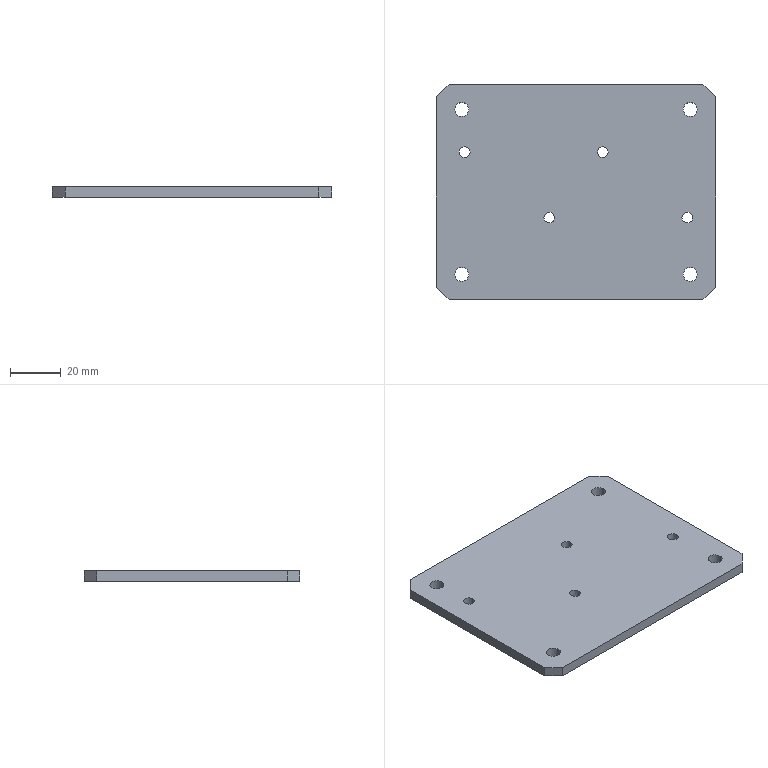Part | SolidWorks | features HoleWzd 2, Chamfer 1, Extrusion 1 | 1 solid | 26 faces | box 110 x 85 x 4 mm | volume 36598 mm3 | cylinder 16 | plane 10 | commonest cylinder face diameters 4.2 x8 5.5 x8
STEP:
#1=CARTESIAN_POINT('',(-45.96,15.733,-2.));
#2=VERTEX_POINT('',#1);
#3=CARTESIAN_POINT('',(-41.76,15.733,-2.));
#4=VERTEX_POINT('',#3);
#5=CARTESIAN_POINT('',(-43.86,15.733,-2.));
#6=DIRECTION('',(0.,0.,1.));
#7=DIRECTION('',(1.,0.,0.));
#8=AXIS2_PLACEMENT_3D('',#5,#6,#7);
#9=CIRCLE('',#8,2.1);
#10=EDGE_CURVE('',#2,#4,#9,.T.);
#11=ORIENTED_EDGE('',*,*,#10,.F.);
#12=CARTESIAN_POINT('',(-45.96,15.733,2.));
#13=VERTEX_POINT('',#12);
#14=CARTESIAN_POINT('',(-45.96,15.733,2.));
#15=DIRECTION('',(0.,0.,1.));
#16=VECTOR('',#15,1000.);
#17=LINE('',#14,#16);
#18=EDGE_CURVE('',#2,#13,#17,.T.);
#19=ORIENTED_EDGE('',*,*,#18,.T.);
#20=CARTESIAN_POINT('',(-41.76,15.733,2.));
#21=VERTEX_POINT('',#20);
#22=CARTESIAN_POINT('',(-43.86,15.733,2.));
#23=DIRECTION('',(0.,0.,1.));
#24=DIRECTION('',(1.,0.,0.));
#25=AXIS2_PLACEMENT_3D('',#22,#23,#24);
#26=CIRCLE('',#25,2.1);
#27=EDGE_CURVE('',#13,#21,#26,.T.);
#28=ORIENTED_EDGE('',*,*,#27,.T.);
#29=CARTESIAN_POINT('',(-41.76,15.733,2.));
#30=DIRECTION('',(0.,0.,1.));
#31=VECTOR('',#30,1000.);
#32=LINE('',#29,#31);
#33=EDGE_CURVE('',#4,#21,#32,.T.);
#34=ORIENTED_EDGE('',*,*,#33,.F.);
#35=EDGE_LOOP('',(#11,#19,#28,#34));
#36=FACE_OUTER_BOUND('',#35,.T.);
#37=CARTESIAN_POINT('',(-43.86,15.733,2.));
#38=DIRECTION('',(0.,0.,1.));
#39=DIRECTION('',(1.,0.,0.));
#40=AXIS2_PLACEMENT_3D('',#37,#38,#39);
#41=CYLINDRICAL_SURFACE('',#40,2.1);
#42=ADVANCED_FACE('',(#36),#41,.F.);
#43=CARTESIAN_POINT('',(8.46,15.733,-2.));
#44=VERTEX_POINT('',#43);
#45=CARTESIAN_POINT('',(12.66,15.733,-2.));
#46=VERTEX_POINT('',#45);
#47=CARTESIAN_POINT('',(10.56,15.733,-2.));
#48=DIRECTION('',(0.,0.,1.));
#49=DIRECTION('',(1.,0.,0.));
#50=AXIS2_PLACEMENT_3D('',#47,#48,#49);
#51=CIRCLE('',#50,2.1);
#52=EDGE_CURVE('',#44,#46,#51,.T.);
#53=ORIENTED_EDGE('',*,*,#52,.F.);
#54=CARTESIAN_POINT('',(8.46,15.733,2.));
#55=VERTEX_POINT('',#54);
#56=CARTESIAN_POINT('',(8.46,15.733,2.));
#57=DIRECTION('',(0.,0.,1.));
#58=VECTOR('',#57,1000.);
#59=LINE('',#56,#58);
#60=EDGE_CURVE('',#44,#55,#59,.T.);
#61=ORIENTED_EDGE('',*,*,#60,.T.);
#62=CARTESIAN_POINT('',(12.66,15.733,2.));
#63=VERTEX_POINT('',#62);
#64=CARTESIAN_POINT('',(10.56,15.733,2.));
#65=DIRECTION('',(0.,0.,1.));
#66=DIRECTION('',(1.,0.,0.));
#67=AXIS2_PLACEMENT_3D('',#64,#65,#66);
#68=CIRCLE('',#67,2.1);
#69=EDGE_CURVE('',#55,#63,#68,.T.);
#70=ORIENTED_EDGE('',*,*,#69,.T.);
#71=CARTESIAN_POINT('',(12.66,15.733,2.));
#72=DIRECTION('',(0.,0.,1.));
#73=VECTOR('',#72,1000.);
#74=LINE('',#71,#73);
#75=EDGE_CURVE('',#46,#63,#74,.T.);
#76=ORIENTED_EDGE('',*,*,#75,.F.);
#77=EDGE_LOOP('',(#53,#61,#70,#76));
#78=FACE_OUTER_BOUND('',#77,.T.);
#79=CARTESIAN_POINT('',(10.56,15.733,2.));
#80=DIRECTION('',(0.,0.,1.));
#81=DIRECTION('',(1.,0.,0.));
#82=AXIS2_PLACEMENT_3D('',#79,#80,#81);
#83=CYLINDRICAL_SURFACE('',#82,2.1);
#84=ADVANCED_FACE('',(#78),#83,.F.);
#85=CARTESIAN_POINT('',(-12.66,-10.077,-2.));
#86=VERTEX_POINT('',#85);
#87=CARTESIAN_POINT('',(-8.46,-10.077,-2.));
#88=VERTEX_POINT('',#87);
#89=CARTESIAN_POINT('',(-10.56,-10.077,-2.));
#90=DIRECTION('',(0.,0.,1.));
#91=DIRECTION('',(1.,0.,0.));
#92=AXIS2_PLACEMENT_3D('',#89,#90,#91);
#93=CIRCLE('',#92,2.1);
#94=EDGE_CURVE('',#86,#88,#93,.T.);
#95=ORIENTED_EDGE('',*,*,#94,.F.);
#96=CARTESIAN_POINT('',(-12.66,-10.077,2.));
#97=VERTEX_POINT('',#96);
#98=CARTESIAN_POINT('',(-12.66,-10.077,2.));
#99=DIRECTION('',(0.,0.,1.));
#100=VECTOR('',#99,1000.);
#101=LINE('',#98,#100);
#102=EDGE_CURVE('',#86,#97,#101,.T.);
#103=ORIENTED_EDGE('',*,*,#102,.T.);
#104=CARTESIAN_POINT('',(-8.46,-10.077,2.));
#105=VERTEX_POINT('',#104);
#106=CARTESIAN_POINT('',(-10.56,-10.077,2.));
#107=DIRECTION('',(0.,0.,1.));
#108=DIRECTION('',(1.,0.,0.));
#109=AXIS2_PLACEMENT_3D('',#106,#107,#108);
#110=CIRCLE('',#109,2.1);
#111=EDGE_CURVE('',#97,#105,#110,.T.);
#112=ORIENTED_EDGE('',*,*,#111,.T.);
#113=CARTESIAN_POINT('',(-8.46,-10.077,2.));
#114=DIRECTION('',(0.,0.,1.));
#115=VECTOR('',#114,1000.);
#116=LINE('',#113,#115);
#117=EDGE_CURVE('',#88,#105,#116,.T.);
#118=ORIENTED_EDGE('',*,*,#117,.F.);
#119=EDGE_LOOP('',(#95,#103,#112,#118));
#120=FACE_OUTER_BOUND('',#119,.T.);
#121=CARTESIAN_POINT('',(-10.56,-10.077,2.));
#122=DIRECTION('',(0.,0.,1.));
#123=DIRECTION('',(1.,0.,0.));
#124=AXIS2_PLACEMENT_3D('',#121,#122,#123);
#125=CYLINDRICAL_SURFACE('',#124,2.1);
#126=ADVANCED_FACE('',(#120),#125,.F.);
#127=CARTESIAN_POINT('',(41.76,-10.077,-2.));
#128=VERTEX_POINT('',#127);
#129=CARTESIAN_POINT('',(45.96,-10.077,-2.));
#130=VERTEX_POINT('',#129);
#131=CARTESIAN_POINT('',(43.86,-10.077,-2.));
#132=DIRECTION('',(0.,0.,1.));
#133=DIRECTION('',(1.,0.,0.));
#134=AXIS2_PLACEMENT_3D('',#131,#132,#133);
#135=CIRCLE('',#134,2.1);
#136=EDGE_CURVE('',#128,#130,#135,.T.);
#137=ORIENTED_EDGE('',*,*,#136,.F.);
#138=CARTESIAN_POINT('',(41.76,-10.077,2.));
#139=VERTEX_POINT('',#138);
#140=CARTESIAN_POINT('',(41.76,-10.077,2.));
#141=DIRECTION('',(0.,0.,1.));
#142=VECTOR('',#141,1000.);
#143=LINE('',#140,#142);
#144=EDGE_CURVE('',#128,#139,#143,.T.);
#145=ORIENTED_EDGE('',*,*,#144,.T.);
#146=CARTESIAN_POINT('',(45.96,-10.077,2.));
#147=VERTEX_POINT('',#146);
#148=CARTESIAN_POINT('',(43.86,-10.077,2.));
#149=DIRECTION('',(0.,0.,1.));
#150=DIRECTION('',(1.,0.,0.));
#151=AXIS2_PLACEMENT_3D('',#148,#149,#150);
#152=CIRCLE('',#151,2.1);
#153=EDGE_CURVE('',#139,#147,#152,.T.);
#154=ORIENTED_EDGE('',*,*,#153,.T.);
#155=CARTESIAN_POINT('',(45.96,-10.077,2.));
#156=DIRECTION('',(0.,0.,1.));
#157=VECTOR('',#156,1000.);
#158=LINE('',#155,#157);
#159=EDGE_CURVE('',#130,#147,#158,.T.);
#160=ORIENTED_EDGE('',*,*,#159,.F.);
#161=EDGE_LOOP('',(#137,#145,#154,#160));
#162=FACE_OUTER_BOUND('',#161,.T.);
#163=CARTESIAN_POINT('',(43.86,-10.077,2.));
#164=DIRECTION('',(0.,0.,1.));
#165=DIRECTION('',(1.,0.,0.));
#166=AXIS2_PLACEMENT_3D('',#163,#164,#165);
#167=CYLINDRICAL_SURFACE('',#166,2.1);
#168=ADVANCED_FACE('',(#162),#167,.F.);
#169=CARTESIAN_POINT('',(42.25,32.5,-2.));
#170=VERTEX_POINT('',#169);
#171=CARTESIAN_POINT('',(47.75,32.5,-2.));
#172=VERTEX_POINT('',#171);
#173=CARTESIAN_POINT('',(45.,32.5,-2.));
#174=DIRECTION('',(0.,0.,1.));
#175=DIRECTION('',(1.,0.,0.));
#176=AXIS2_PLACEMENT_3D('',#173,#174,#175);
#177=CIRCLE('',#176,2.75);
#178=EDGE_CURVE('',#170,#172,#177,.T.);
#179=ORIENTED_EDGE('',*,*,#178,.F.);
#180=CARTESIAN_POINT('',(42.25,32.5,2.));
#181=VERTEX_POINT('',#180);
#182=CARTESIAN_POINT('',(42.25,32.5,2.));
#183=DIRECTION('',(0.,0.,1.));
#184=VECTOR('',#183,1000.);
#185=LINE('',#182,#184);
#186=EDGE_CURVE('',#170,#181,#185,.T.);
#187=ORIENTED_EDGE('',*,*,#186,.T.);
#188=CARTESIAN_POINT('',(47.75,32.5,2.));
#189=VERTEX_POINT('',#188);
#190=CARTESIAN_POINT('',(45.,32.5,2.));
#191=DIRECTION('',(0.,0.,1.));
#192=DIRECTION('',(1.,0.,0.));
#193=AXIS2_PLACEMENT_3D('',#190,#191,#192);
#194=CIRCLE('',#193,2.75);
#195=EDGE_CURVE('',#181,#189,#194,.T.);
#196=ORIENTED_EDGE('',*,*,#195,.T.);
#197=CARTESIAN_POINT('',(47.75,32.5,2.));
#198=DIRECTION('',(0.,0.,1.));
#199=VECTOR('',#198,1000.);
#200=LINE('',#197,#199);
#201=EDGE_CURVE('',#172,#189,#200,.T.);
#202=ORIENTED_EDGE('',*,*,#201,.F.);
#203=EDGE_LOOP('',(#179,#187,#196,#202));
#204=FACE_OUTER_BOUND('',#203,.T.);
#205=CARTESIAN_POINT('',(45.,32.5,2.));
#206=DIRECTION('',(0.,0.,1.));
#207=DIRECTION('',(1.,0.,0.));
#208=AXIS2_PLACEMENT_3D('',#205,#206,#207);
#209=CYLINDRICAL_SURFACE('',#208,2.75);
#210=ADVANCED_FACE('',(#204),#209,.F.);
#211=CARTESIAN_POINT('',(42.25,-32.5,-2.));
#212=VERTEX_POINT('',#211);
#213=CARTESIAN_POINT('',(47.75,-32.5,-2.));
#214=VERTEX_POINT('',#213);
#215=CARTESIAN_POINT('',(45.,-32.5,-2.));
#216=DIRECTION('',(0.,0.,1.));
#217=DIRECTION('',(1.,0.,0.));
#218=AXIS2_PLACEMENT_3D('',#215,#216,#217);
#219=CIRCLE('',#218,2.75);
#220=EDGE_CURVE('',#212,#214,#219,.T.);
#221=ORIENTED_EDGE('',*,*,#220,.F.);
#222=CARTESIAN_POINT('',(42.25,-32.5,2.));
#223=VERTEX_POINT('',#222);
#224=CARTESIAN_POINT('',(42.25,-32.5,2.));
#225=DIRECTION('',(0.,0.,1.));
#226=VECTOR('',#225,1000.);
#227=LINE('',#224,#226);
#228=EDGE_CURVE('',#212,#223,#227,.T.);
#229=ORIENTED_EDGE('',*,*,#228,.T.);
#230=CARTESIAN_POINT('',(47.75,-32.5,2.));
#231=VERTEX_POINT('',#230);
#232=CARTESIAN_POINT('',(45.,-32.5,2.));
#233=DIRECTION('',(0.,0.,1.));
#234=DIRECTION('',(1.,0.,0.));
#235=AXIS2_PLACEMENT_3D('',#232,#233,#234);
#236=CIRCLE('',#235,2.75);
#237=EDGE_CURVE('',#223,#231,#236,.T.);
#238=ORIENTED_EDGE('',*,*,#237,.T.);
#239=CARTESIAN_POINT('',(47.75,-32.5,2.));
#240=DIRECTION('',(0.,0.,1.));
#241=VECTOR('',#240,1000.);
#242=LINE('',#239,#241);
#243=EDGE_CURVE('',#214,#231,#242,.T.);
#244=ORIENTED_EDGE('',*,*,#243,.F.);
#245=EDGE_LOOP('',(#221,#229,#238,#244));
#246=FACE_OUTER_BOUND('',#245,.T.);
#247=CARTESIAN_POINT('',(45.,-32.5,2.));
#248=DIRECTION('',(0.,0.,1.));
#249=DIRECTION('',(1.,0.,0.));
#250=AXIS2_PLACEMENT_3D('',#247,#248,#249);
#251=CYLINDRICAL_SURFACE('',#250,2.75);
#252=ADVANCED_FACE('',(#246),#251,.F.);
#253=CARTESIAN_POINT('',(-47.75,-32.5,-2.));
#254=VERTEX_POINT('',#253);
#255=CARTESIAN_POINT('',(-42.25,-32.5,-2.));
#256=VERTEX_POINT('',#255);
#257=CARTESIAN_POINT('',(-45.,-32.5,-2.));
#258=DIRECTION('',(0.,0.,1.));
#259=DIRECTION('',(1.,0.,0.));
#260=AXIS2_PLACEMENT_3D('',#257,#258,#259);
#261=CIRCLE('',#260,2.75);
#262=EDGE_CURVE('',#254,#256,#261,.T.);
#263=ORIENTED_EDGE('',*,*,#262,.F.);
#264=CARTESIAN_POINT('',(-47.75,-32.5,2.));
#265=VERTEX_POINT('',#264);
#266=CARTESIAN_POINT('',(-47.75,-32.5,2.));
#267=DIRECTION('',(0.,0.,1.));
#268=VECTOR('',#267,1000.);
#269=LINE('',#266,#268);
#270=EDGE_CURVE('',#254,#265,#269,.T.);
#271=ORIENTED_EDGE('',*,*,#270,.T.);
#272=CARTESIAN_POINT('',(-42.25,-32.5,2.));
#273=VERTEX_POINT('',#272);
#274=CARTESIAN_POINT('',(-45.,-32.5,2.));
#275=DIRECTION('',(0.,0.,1.));
#276=DIRECTION('',(1.,0.,0.));
#277=AXIS2_PLACEMENT_3D('',#274,#275,#276);
#278=CIRCLE('',#277,2.75);
#279=EDGE_CURVE('',#265,#273,#278,.T.);
#280=ORIENTED_EDGE('',*,*,#279,.T.);
#281=CARTESIAN_POINT('',(-42.25,-32.5,2.));
#282=DIRECTION('',(0.,0.,1.));
#283=VECTOR('',#282,1000.);
#284=LINE('',#281,#283);
#285=EDGE_CURVE('',#256,#273,#284,.T.);
#286=ORIENTED_EDGE('',*,*,#285,.F.);
#287=EDGE_LOOP('',(#263,#271,#280,#286));
#288=FACE_OUTER_BOUND('',#287,.T.);
#289=CARTESIAN_POINT('',(-45.,-32.5,2.));
#290=DIRECTION('',(0.,0.,1.));
#291=DIRECTION('',(1.,0.,0.));
#292=AXIS2_PLACEMENT_3D('',#289,#290,#291);
#293=CYLINDRICAL_SURFACE('',#292,2.75);
#294=ADVANCED_FACE('',(#288),#293,.F.);
#295=CARTESIAN_POINT('',(-47.75,32.5,-2.));
#296=VERTEX_POINT('',#295);
#297=CARTESIAN_POINT('',(-42.25,32.5,-2.));
#298=VERTEX_POINT('',#297);
#299=CARTESIAN_POINT('',(-45.,32.5,-2.));
#300=DIRECTION('',(0.,0.,1.));
#301=DIRECTION('',(1.,0.,0.));
#302=AXIS2_PLACEMENT_3D('',#299,#300,#301);
#303=CIRCLE('',#302,2.75);
#304=EDGE_CURVE('',#296,#298,#303,.T.);
#305=ORIENTED_EDGE('',*,*,#304,.F.);
#306=CARTESIAN_POINT('',(-47.75,32.5,2.));
#307=VERTEX_POINT('',#306);
#308=CARTESIAN_POINT('',(-47.75,32.5,2.));
#309=DIRECTION('',(0.,0.,1.));
#310=VECTOR('',#309,1000.);
#311=LINE('',#308,#310);
#312=EDGE_CURVE('',#296,#307,#311,.T.);
#313=ORIENTED_EDGE('',*,*,#312,.T.);
#314=CARTESIAN_POINT('',(-42.25,32.5,2.));
#315=VERTEX_POINT('',#314);
#316=CARTESIAN_POINT('',(-45.,32.5,2.));
#317=DIRECTION('',(0.,0.,1.));
#318=DIRECTION('',(1.,0.,0.));
#319=AXIS2_PLACEMENT_3D('',#316,#317,#318);
#320=CIRCLE('',#319,2.75);
#321=EDGE_CURVE('',#307,#315,#320,.T.);
#322=ORIENTED_EDGE('',*,*,#321,.T.);
#323=CARTESIAN_POINT('',(-42.25,32.5,2.));
#324=DIRECTION('',(0.,0.,1.));
#325=VECTOR('',#324,1000.);
#326=LINE('',#323,#325);
#327=EDGE_CURVE('',#298,#315,#326,.T.);
#328=ORIENTED_EDGE('',*,*,#327,.F.);
#329=EDGE_LOOP('',(#305,#313,#322,#328));
#330=FACE_OUTER_BOUND('',#329,.T.);
#331=CARTESIAN_POINT('',(-45.,32.5,2.));
#332=DIRECTION('',(0.,0.,1.));
#333=DIRECTION('',(1.,0.,0.));
#334=AXIS2_PLACEMENT_3D('',#331,#332,#333);
#335=CYLINDRICAL_SURFACE('',#334,2.75);
#336=ADVANCED_FACE('',(#330),#335,.F.);
#337=CARTESIAN_POINT('',(-55.,37.5,2.));
#338=VERTEX_POINT('',#337);
#339=CARTESIAN_POINT('',(-55.,-37.5,2.));
#340=VERTEX_POINT('',#339);
#341=CARTESIAN_POINT('',(-55.,42.5,2.));
#342=DIRECTION('',(0.,-1.,0.));
#343=VECTOR('',#342,1000.);
#344=LINE('',#341,#343);
#345=EDGE_CURVE('',#338,#340,#344,.T.);
#346=ORIENTED_EDGE('',*,*,#345,.F.);
#347=CARTESIAN_POINT('',(-55.,37.5,-2.));
#348=VERTEX_POINT('',#347);
#349=CARTESIAN_POINT('',(-55.,37.5,2.));
#350=DIRECTION('',(0.,0.,-1.));
#351=VECTOR('',#350,1000.);
#352=LINE('',#349,#351);
#353=EDGE_CURVE('',#338,#348,#352,.T.);
#354=ORIENTED_EDGE('',*,*,#353,.T.);
#355=CARTESIAN_POINT('',(-55.,-37.5,-2.));
#356=VERTEX_POINT('',#355);
#357=CARTESIAN_POINT('',(-55.,42.5,-2.));
#358=DIRECTION('',(0.,-1.,0.));
#359=VECTOR('',#358,1000.);
#360=LINE('',#357,#359);
#361=EDGE_CURVE('',#348,#356,#360,.T.);
#362=ORIENTED_EDGE('',*,*,#361,.T.);
#363=CARTESIAN_POINT('',(-55.,-37.5,2.));
#364=DIRECTION('',(0.,0.,1.));
#365=VECTOR('',#364,1000.);
#366=LINE('',#363,#365);
#367=EDGE_CURVE('',#356,#340,#366,.T.);
#368=ORIENTED_EDGE('',*,*,#367,.T.);
#369=EDGE_LOOP('',(#346,#354,#362,#368));
#370=FACE_OUTER_BOUND('',#369,.T.);
#371=CARTESIAN_POINT('',(-55.,42.5,2.));
#372=DIRECTION('',(1.,0.,0.));
#373=DIRECTION('',(0.,0.,-1.));
#374=AXIS2_PLACEMENT_3D('',#371,#372,#373);
#375=PLANE('',#374);
#376=ADVANCED_FACE('',(#370),#375,.F.);
#377=CARTESIAN_POINT('',(-50.,-42.5,-2.));
#378=VERTEX_POINT('',#377);
#379=CARTESIAN_POINT('',(50.,-42.5,-2.));
#380=VERTEX_POINT('',#379);
#381=CARTESIAN_POINT('',(-55.,-42.5,-2.));
#382=DIRECTION('',(1.,0.,0.));
#383=VECTOR('',#382,1000.);
#384=LINE('',#381,#383);
#385=EDGE_CURVE('',#378,#380,#384,.T.);
#386=ORIENTED_EDGE('',*,*,#385,.T.);
#387=CARTESIAN_POINT('',(50.,-42.5,2.));
#388=VERTEX_POINT('',#387);
#389=CARTESIAN_POINT('',(50.,-42.5,2.));
#390=DIRECTION('',(0.,0.,1.));
#391=VECTOR('',#390,1000.);
#392=LINE('',#389,#391);
#393=EDGE_CURVE('',#380,#388,#392,.T.);
#394=ORIENTED_EDGE('',*,*,#393,.T.);
#395=CARTESIAN_POINT('',(-50.,-42.5,2.));
#396=VERTEX_POINT('',#395);
#397=CARTESIAN_POINT('',(-55.,-42.5,2.));
#398=DIRECTION('',(1.,0.,0.));
#399=VECTOR('',#398,1000.);
#400=LINE('',#397,#399);
#401=EDGE_CURVE('',#396,#388,#400,.T.);
#402=ORIENTED_EDGE('',*,*,#401,.F.);
#403=CARTESIAN_POINT('',(-50.,-42.5,2.));
#404=DIRECTION('',(0.,0.,-1.));
#405=VECTOR('',#404,1000.);
#406=LINE('',#403,#405);
#407=EDGE_CURVE('',#396,#378,#406,.T.);
#408=ORIENTED_EDGE('',*,*,#407,.T.);
#409=EDGE_LOOP('',(#386,#394,#402,#408));
#410=FACE_OUTER_BOUND('',#409,.T.);
#411=CARTESIAN_POINT('',(-55.,-42.5,2.));
#412=DIRECTION('',(0.,1.,0.));
#413=DIRECTION('',(0.,0.,1.));
#414=AXIS2_PLACEMENT_3D('',#411,#412,#413);
#415=PLANE('',#414);
#416=ADVANCED_FACE('',(#410),#415,.F.);
#417=CARTESIAN_POINT('',(55.,-37.5,-2.));
#418=VERTEX_POINT('',#417);
#419=CARTESIAN_POINT('',(55.,37.5,-2.));
#420=VERTEX_POINT('',#419);
#421=CARTESIAN_POINT('',(55.,42.5,-2.));
#422=DIRECTION('',(0.,1.,0.));
#423=VECTOR('',#422,1000.);
#424=LINE('',#421,#423);
#425=EDGE_CURVE('',#418,#420,#424,.T.);
#426=ORIENTED_EDGE('',*,*,#425,.T.);
#427=CARTESIAN_POINT('',(55.,37.5,2.));
#428=VERTEX_POINT('',#427);
#429=CARTESIAN_POINT('',(55.,37.5,2.));
#430=DIRECTION('',(0.,0.,1.));
#431=VECTOR('',#430,1000.);
#432=LINE('',#429,#431);
#433=EDGE_CURVE('',#420,#428,#432,.T.);
#434=ORIENTED_EDGE('',*,*,#433,.T.);
#435=CARTESIAN_POINT('',(55.,-37.5,2.));
#436=VERTEX_POINT('',#435);
#437=CARTESIAN_POINT('',(55.,42.5,2.));
#438=DIRECTION('',(0.,1.,0.));
#439=VECTOR('',#438,1000.);
#440=LINE('',#437,#439);
#441=EDGE_CURVE('',#436,#428,#440,.T.);
#442=ORIENTED_EDGE('',*,*,#441,.F.);
#443=CARTESIAN_POINT('',(55.,-37.5,2.));
#444=DIRECTION('',(0.,0.,-1.));
#445=VECTOR('',#444,1000.);
#446=LINE('',#443,#445);
#447=EDGE_CURVE('',#436,#418,#446,.T.);
#448=ORIENTED_EDGE('',*,*,#447,.T.);
#449=EDGE_LOOP('',(#426,#434,#442,#448));
#450=FACE_OUTER_BOUND('',#449,.T.);
#451=CARTESIAN_POINT('',(55.,42.5,2.));
#452=DIRECTION('',(-1.,0.,0.));
#453=DIRECTION('',(0.,0.,1.));
#454=AXIS2_PLACEMENT_3D('',#451,#452,#453);
#455=PLANE('',#454);
#456=ADVANCED_FACE('',(#450),#455,.F.);
#457=CARTESIAN_POINT('',(50.,42.5,-2.));
#458=VERTEX_POINT('',#457);
#459=CARTESIAN_POINT('',(-50.,42.5,-2.));
#460=VERTEX_POINT('',#459);
#461=CARTESIAN_POINT('',(-55.,42.5,-2.));
#462=DIRECTION('',(-1.,0.,0.));
#463=VECTOR('',#462,1000.);
#464=LINE('',#461,#463);
#465=EDGE_CURVE('',#458,#460,#464,.T.);
#466=ORIENTED_EDGE('',*,*,#465,.T.);
#467=CARTESIAN_POINT('',(-50.,42.5,2.));
#468=VERTEX_POINT('',#467);
#469=CARTESIAN_POINT('',(-50.,42.5,2.));
#470=DIRECTION('',(0.,0.,1.));
#471=VECTOR('',#470,1000.);
#472=LINE('',#469,#471);
#473=EDGE_CURVE('',#460,#468,#472,.T.);
#474=ORIENTED_EDGE('',*,*,#473,.T.);
#475=CARTESIAN_POINT('',(50.,42.5,2.));
#476=VERTEX_POINT('',#475);
#477=CARTESIAN_POINT('',(-55.,42.5,2.));
#478=DIRECTION('',(-1.,0.,0.));
#479=VECTOR('',#478,1000.);
#480=LINE('',#477,#479);
#481=EDGE_CURVE('',#476,#468,#480,.T.);
#482=ORIENTED_EDGE('',*,*,#481,.F.);
#483=CARTESIAN_POINT('',(50.,42.5,2.));
#484=DIRECTION('',(0.,0.,-1.));
#485=VECTOR('',#484,1000.);
#486=LINE('',#483,#485);
#487=EDGE_CURVE('',#476,#458,#486,.T.);
#488=ORIENTED_EDGE('',*,*,#487,.T.);
#489=EDGE_LOOP('',(#466,#474,#482,#488));
#490=FACE_OUTER_BOUND('',#489,.T.);
#491=CARTESIAN_POINT('',(-55.,42.5,2.));
#492=DIRECTION('',(0.,-1.,0.));
#493=DIRECTION('',(0.,0.,-1.));
#494=AXIS2_PLACEMENT_3D('',#491,#492,#493);
#495=PLANE('',#494);
#496=ADVANCED_FACE('',(#490),#495,.F.);
#497=CARTESIAN_POINT('',(-43.86,15.733,2.));
#498=DIRECTION('',(0.,0.,1.));
#499=DIRECTION('',(1.,0.,0.));
#500=AXIS2_PLACEMENT_3D('',#497,#498,#499);
#501=CIRCLE('',#500,2.1);
#502=EDGE_CURVE('',#21,#13,#501,.T.);
#503=ORIENTED_EDGE('',*,*,#502,.F.);
#504=ORIENTED_EDGE('',*,*,#27,.F.);
#505=EDGE_LOOP('',(#503,#504));
#506=FACE_BOUND('',#505,.T.);
#507=CARTESIAN_POINT('',(10.56,15.733,2.));
#508=DIRECTION('',(0.,0.,1.));
#509=DIRECTION('',(1.,0.,0.));
#510=AXIS2_PLACEMENT_3D('',#507,#508,#509);
#511=CIRCLE('',#510,2.1);
#512=EDGE_CURVE('',#63,#55,#511,.T.);
#513=ORIENTED_EDGE('',*,*,#512,.F.);
#514=ORIENTED_EDGE('',*,*,#69,.F.);
#515=EDGE_LOOP('',(#513,#514));
#516=FACE_BOUND('',#515,.T.);
#517=CARTESIAN_POINT('',(-10.56,-10.077,2.));
#518=DIRECTION('',(0.,0.,1.));
#519=DIRECTION('',(1.,0.,0.));
#520=AXIS2_PLACEMENT_3D('',#517,#518,#519);
#521=CIRCLE('',#520,2.1);
#522=EDGE_CURVE('',#105,#97,#521,.T.);
#523=ORIENTED_EDGE('',*,*,#522,.F.);
#524=ORIENTED_EDGE('',*,*,#111,.F.);
#525=EDGE_LOOP('',(#523,#524));
#526=FACE_BOUND('',#525,.T.);
#527=CARTESIAN_POINT('',(43.86,-10.077,2.));
#528=DIRECTION('',(0.,0.,1.));
#529=DIRECTION('',(1.,0.,0.));
#530=AXIS2_PLACEMENT_3D('',#527,#528,#529);
#531=CIRCLE('',#530,2.1);
#532=EDGE_CURVE('',#147,#139,#531,.T.);
#533=ORIENTED_EDGE('',*,*,#532,.F.);
#534=ORIENTED_EDGE('',*,*,#153,.F.);
#535=EDGE_LOOP('',(#533,#534));
#536=FACE_BOUND('',#535,.T.);
#537=CARTESIAN_POINT('',(45.,32.5,2.));
#538=DIRECTION('',(0.,0.,1.));
#539=DIRECTION('',(1.,0.,0.));
#540=AXIS2_PLACEMENT_3D('',#537,#538,#539);
#541=CIRCLE('',#540,2.75);
#542=EDGE_CURVE('',#189,#181,#541,.T.);
#543=ORIENTED_EDGE('',*,*,#542,.F.);
#544=ORIENTED_EDGE('',*,*,#195,.F.);
#545=EDGE_LOOP('',(#543,#544));
#546=FACE_BOUND('',#545,.T.);
#547=CARTESIAN_POINT('',(45.,-32.5,2.));
#548=DIRECTION('',(0.,0.,1.));
#549=DIRECTION('',(1.,0.,0.));
#550=AXIS2_PLACEMENT_3D('',#547,#548,#549);
#551=CIRCLE('',#550,2.75);
#552=EDGE_CURVE('',#231,#223,#551,.T.);
#553=ORIENTED_EDGE('',*,*,#552,.F.);
#554=ORIENTED_EDGE('',*,*,#237,.F.);
#555=EDGE_LOOP('',(#553,#554));
#556=FACE_BOUND('',#555,.T.);
#557=CARTESIAN_POINT('',(-45.,-32.5,2.));
#558=DIRECTION('',(0.,0.,1.));
#559=DIRECTION('',(1.,0.,0.));
#560=AXIS2_PLACEMENT_3D('',#557,#558,#559);
#561=CIRCLE('',#560,2.75);
#562=EDGE_CURVE('',#273,#265,#561,.T.);
#563=ORIENTED_EDGE('',*,*,#562,.F.);
#564=ORIENTED_EDGE('',*,*,#279,.F.);
#565=EDGE_LOOP('',(#563,#564));
#566=FACE_BOUND('',#565,.T.);
#567=CARTESIAN_POINT('',(-45.,32.5,2.));
#568=DIRECTION('',(0.,0.,1.));
#569=DIRECTION('',(1.,0.,0.));
#570=AXIS2_PLACEMENT_3D('',#567,#568,#569);
#571=CIRCLE('',#570,2.75);
#572=EDGE_CURVE('',#315,#307,#571,.T.);
#573=ORIENTED_EDGE('',*,*,#572,.F.);
#574=ORIENTED_EDGE('',*,*,#321,.F.);
#575=EDGE_LOOP('',(#573,#574));
#576=FACE_BOUND('',#575,.T.);
#577=ORIENTED_EDGE('',*,*,#481,.T.);
#578=CARTESIAN_POINT('',(-46.25,46.25,2.));
#579=DIRECTION('',(-0.7071,-0.7071,0.));
#580=VECTOR('',#579,1000.);
#581=LINE('',#578,#580);
#582=EDGE_CURVE('',#468,#338,#581,.T.);
#583=ORIENTED_EDGE('',*,*,#582,.T.);
#584=ORIENTED_EDGE('',*,*,#345,.T.);
#585=CARTESIAN_POINT('',(-46.25,-46.25,2.));
#586=DIRECTION('',(0.7071,-0.7071,0.));
#587=VECTOR('',#586,1000.);
#588=LINE('',#585,#587);
#589=EDGE_CURVE('',#340,#396,#588,.T.);
#590=ORIENTED_EDGE('',*,*,#589,.T.);
#591=ORIENTED_EDGE('',*,*,#401,.T.);
#592=CARTESIAN_POINT('',(46.25,-46.25,2.));
#593=DIRECTION('',(0.7071,0.7071,0.));
#594=VECTOR('',#593,1000.);
#595=LINE('',#592,#594);
#596=EDGE_CURVE('',#388,#436,#595,.T.);
#597=ORIENTED_EDGE('',*,*,#596,.T.);
#598=ORIENTED_EDGE('',*,*,#441,.T.);
#599=CARTESIAN_POINT('',(46.25,46.25,2.));
#600=DIRECTION('',(-0.7071,0.7071,0.));
#601=VECTOR('',#600,1000.);
#602=LINE('',#599,#601);
#603=EDGE_CURVE('',#428,#476,#602,.T.);
#604=ORIENTED_EDGE('',*,*,#603,.T.);
#605=EDGE_LOOP('',(#577,#583,#584,#590,#591,#597,#598,#604));
#606=FACE_OUTER_BOUND('',#605,.T.);
#607=CARTESIAN_POINT('',(0.,0.,2.));
#608=DIRECTION('',(0.,0.,1.));
#609=DIRECTION('',(1.,0.,0.));
#610=AXIS2_PLACEMENT_3D('',#607,#608,#609);
#611=PLANE('',#610);
#612=ADVANCED_FACE('',(#506,#516,#526,#536,#546,#556,#566,#576,#606),#611,.T.);
#613=CARTESIAN_POINT('',(-43.86,15.733,-2.));
#614=DIRECTION('',(0.,0.,1.));
#615=DIRECTION('',(1.,0.,0.));
#616=AXIS2_PLACEMENT_3D('',#613,#614,#615);
#617=CIRCLE('',#616,2.1);
#618=EDGE_CURVE('',#4,#2,#617,.T.);
#619=ORIENTED_EDGE('',*,*,#618,.T.);
#620=ORIENTED_EDGE('',*,*,#10,.T.);
#621=EDGE_LOOP('',(#619,#620));
#622=FACE_BOUND('',#621,.T.);
#623=CARTESIAN_POINT('',(10.56,15.733,-2.));
#624=DIRECTION('',(0.,0.,1.));
#625=DIRECTION('',(1.,0.,0.));
#626=AXIS2_PLACEMENT_3D('',#623,#624,#625);
#627=CIRCLE('',#626,2.1);
#628=EDGE_CURVE('',#46,#44,#627,.T.);
#629=ORIENTED_EDGE('',*,*,#628,.T.);
#630=ORIENTED_EDGE('',*,*,#52,.T.);
#631=EDGE_LOOP('',(#629,#630));
#632=FACE_BOUND('',#631,.T.);
#633=CARTESIAN_POINT('',(-10.56,-10.077,-2.));
#634=DIRECTION('',(0.,0.,1.));
#635=DIRECTION('',(1.,0.,0.));
#636=AXIS2_PLACEMENT_3D('',#633,#634,#635);
#637=CIRCLE('',#636,2.1);
#638=EDGE_CURVE('',#88,#86,#637,.T.);
#639=ORIENTED_EDGE('',*,*,#638,.T.);
#640=ORIENTED_EDGE('',*,*,#94,.T.);
#641=EDGE_LOOP('',(#639,#640));
#642=FACE_BOUND('',#641,.T.);
#643=CARTESIAN_POINT('',(43.86,-10.077,-2.));
#644=DIRECTION('',(0.,0.,1.));
#645=DIRECTION('',(1.,0.,0.));
#646=AXIS2_PLACEMENT_3D('',#643,#644,#645);
#647=CIRCLE('',#646,2.1);
#648=EDGE_CURVE('',#130,#128,#647,.T.);
#649=ORIENTED_EDGE('',*,*,#648,.T.);
#650=ORIENTED_EDGE('',*,*,#136,.T.);
#651=EDGE_LOOP('',(#649,#650));
#652=FACE_BOUND('',#651,.T.);
#653=CARTESIAN_POINT('',(45.,32.5,-2.));
#654=DIRECTION('',(0.,0.,1.));
#655=DIRECTION('',(1.,0.,0.));
#656=AXIS2_PLACEMENT_3D('',#653,#654,#655);
#657=CIRCLE('',#656,2.75);
#658=EDGE_CURVE('',#172,#170,#657,.T.);
#659=ORIENTED_EDGE('',*,*,#658,.T.);
#660=ORIENTED_EDGE('',*,*,#178,.T.);
#661=EDGE_LOOP('',(#659,#660));
#662=FACE_BOUND('',#661,.T.);
#663=CARTESIAN_POINT('',(45.,-32.5,-2.));
#664=DIRECTION('',(0.,0.,1.));
#665=DIRECTION('',(1.,0.,0.));
#666=AXIS2_PLACEMENT_3D('',#663,#664,#665);
#667=CIRCLE('',#666,2.75);
#668=EDGE_CURVE('',#214,#212,#667,.T.);
#669=ORIENTED_EDGE('',*,*,#668,.T.);
#670=ORIENTED_EDGE('',*,*,#220,.T.);
#671=EDGE_LOOP('',(#669,#670));
#672=FACE_BOUND('',#671,.T.);
#673=CARTESIAN_POINT('',(-45.,-32.5,-2.));
#674=DIRECTION('',(0.,0.,1.));
#675=DIRECTION('',(1.,0.,0.));
#676=AXIS2_PLACEMENT_3D('',#673,#674,#675);
#677=CIRCLE('',#676,2.75);
#678=EDGE_CURVE('',#256,#254,#677,.T.);
#679=ORIENTED_EDGE('',*,*,#678,.T.);
#680=ORIENTED_EDGE('',*,*,#262,.T.);
#681=EDGE_LOOP('',(#679,#680));
#682=FACE_BOUND('',#681,.T.);
#683=CARTESIAN_POINT('',(-45.,32.5,-2.));
#684=DIRECTION('',(0.,0.,1.));
#685=DIRECTION('',(1.,0.,0.));
#686=AXIS2_PLACEMENT_3D('',#683,#684,#685);
#687=CIRCLE('',#686,2.75);
#688=EDGE_CURVE('',#298,#296,#687,.T.);
#689=ORIENTED_EDGE('',*,*,#688,.T.);
#690=ORIENTED_EDGE('',*,*,#304,.T.);
#691=EDGE_LOOP('',(#689,#690));
#692=FACE_BOUND('',#691,.T.);
#693=ORIENTED_EDGE('',*,*,#361,.F.);
#694=CARTESIAN_POINT('',(-55.,37.5,-2.));
#695=DIRECTION('',(0.7071,0.7071,0.));
#696=VECTOR('',#695,1000.);
#697=LINE('',#694,#696);
#698=EDGE_CURVE('',#348,#460,#697,.T.);
#699=ORIENTED_EDGE('',*,*,#698,.T.);
#700=ORIENTED_EDGE('',*,*,#465,.F.);
#701=CARTESIAN_POINT('',(50.,42.5,-2.));
#702=DIRECTION('',(0.7071,-0.7071,0.));
#703=VECTOR('',#702,1000.);
#704=LINE('',#701,#703);
#705=EDGE_CURVE('',#458,#420,#704,.T.);
#706=ORIENTED_EDGE('',*,*,#705,.T.);
#707=ORIENTED_EDGE('',*,*,#425,.F.);
#708=CARTESIAN_POINT('',(55.,-37.5,-2.));
#709=DIRECTION('',(-0.7071,-0.7071,0.));
#710=VECTOR('',#709,1000.);
#711=LINE('',#708,#710);
#712=EDGE_CURVE('',#418,#380,#711,.T.);
#713=ORIENTED_EDGE('',*,*,#712,.T.);
#714=ORIENTED_EDGE('',*,*,#385,.F.);
#715=CARTESIAN_POINT('',(-50.,-42.5,-2.));
#716=DIRECTION('',(-0.7071,0.7071,0.));
#717=VECTOR('',#716,1000.);
#718=LINE('',#715,#717);
#719=EDGE_CURVE('',#378,#356,#718,.T.);
#720=ORIENTED_EDGE('',*,*,#719,.T.);
#721=EDGE_LOOP('',(#693,#699,#700,#706,#707,#713,#714,#720));
#722=FACE_OUTER_BOUND('',#721,.T.);
#723=CARTESIAN_POINT('',(0.,0.,-2.));
#724=DIRECTION('',(0.,0.,1.));
#725=DIRECTION('',(1.,0.,0.));
#726=AXIS2_PLACEMENT_3D('',#723,#724,#725);
#727=PLANE('',#726);
#728=ADVANCED_FACE('',(#622,#632,#642,#652,#662,#672,#682,#692,#722),#727,.F.);
#729=ORIENTED_EDGE('',*,*,#582,.F.);
#730=ORIENTED_EDGE('',*,*,#473,.F.);
#731=ORIENTED_EDGE('',*,*,#698,.F.);
#732=ORIENTED_EDGE('',*,*,#353,.F.);
#733=EDGE_LOOP('',(#729,#730,#731,#732));
#734=FACE_OUTER_BOUND('',#733,.T.);
#735=CARTESIAN_POINT('',(-55.,37.5,2.));
#736=DIRECTION('',(0.7071,-0.7071,0.));
#737=DIRECTION('',(0.,0.,-1.));
#738=AXIS2_PLACEMENT_3D('',#735,#736,#737);
#739=PLANE('',#738);
#740=ADVANCED_FACE('',(#734),#739,.F.);
#741=ORIENTED_EDGE('',*,*,#603,.F.);
#742=ORIENTED_EDGE('',*,*,#433,.F.);
#743=ORIENTED_EDGE('',*,*,#705,.F.);
#744=ORIENTED_EDGE('',*,*,#487,.F.);
#745=EDGE_LOOP('',(#741,#742,#743,#744));
#746=FACE_OUTER_BOUND('',#745,.T.);
#747=CARTESIAN_POINT('',(50.,42.5,2.));
#748=DIRECTION('',(-0.7071,-0.7071,0.));
#749=DIRECTION('',(0.,0.,-1.));
#750=AXIS2_PLACEMENT_3D('',#747,#748,#749);
#751=PLANE('',#750);
#752=ADVANCED_FACE('',(#746),#751,.F.);
#753=ORIENTED_EDGE('',*,*,#596,.F.);
#754=ORIENTED_EDGE('',*,*,#393,.F.);
#755=ORIENTED_EDGE('',*,*,#712,.F.);
#756=ORIENTED_EDGE('',*,*,#447,.F.);
#757=EDGE_LOOP('',(#753,#754,#755,#756));
#758=FACE_OUTER_BOUND('',#757,.T.);
#759=CARTESIAN_POINT('',(55.,-37.5,2.));
#760=DIRECTION('',(-0.7071,0.7071,0.));
#761=DIRECTION('',(0.,0.,-1.));
#762=AXIS2_PLACEMENT_3D('',#759,#760,#761);
#763=PLANE('',#762);
#764=ADVANCED_FACE('',(#758),#763,.F.);
#765=ORIENTED_EDGE('',*,*,#589,.F.);
#766=ORIENTED_EDGE('',*,*,#367,.F.);
#767=ORIENTED_EDGE('',*,*,#719,.F.);
#768=ORIENTED_EDGE('',*,*,#407,.F.);
#769=EDGE_LOOP('',(#765,#766,#767,#768));
#770=FACE_OUTER_BOUND('',#769,.T.);
#771=CARTESIAN_POINT('',(-50.,-42.5,2.));
#772=DIRECTION('',(0.7071,0.7071,0.));
#773=DIRECTION('',(0.,0.,-1.));
#774=AXIS2_PLACEMENT_3D('',#771,#772,#773);
#775=PLANE('',#774);
#776=ADVANCED_FACE('',(#770),#775,.F.);
#777=ORIENTED_EDGE('',*,*,#312,.F.);
#778=ORIENTED_EDGE('',*,*,#688,.F.);
#779=ORIENTED_EDGE('',*,*,#327,.T.);
#780=ORIENTED_EDGE('',*,*,#572,.T.);
#781=EDGE_LOOP('',(#777,#778,#779,#780));
#782=FACE_OUTER_BOUND('',#781,.T.);
#783=CARTESIAN_POINT('',(-45.,32.5,2.));
#784=DIRECTION('',(0.,0.,1.));
#785=DIRECTION('',(1.,0.,0.));
#786=AXIS2_PLACEMENT_3D('',#783,#784,#785);
#787=CYLINDRICAL_SURFACE('',#786,2.75);
#788=ADVANCED_FACE('',(#782),#787,.F.);
#789=ORIENTED_EDGE('',*,*,#270,.F.);
#790=ORIENTED_EDGE('',*,*,#678,.F.);
#791=ORIENTED_EDGE('',*,*,#285,.T.);
#792=ORIENTED_EDGE('',*,*,#562,.T.);
#793=EDGE_LOOP('',(#789,#790,#791,#792));
#794=FACE_OUTER_BOUND('',#793,.T.);
#795=CARTESIAN_POINT('',(-45.,-32.5,2.));
#796=DIRECTION('',(0.,0.,1.));
#797=DIRECTION('',(1.,0.,0.));
#798=AXIS2_PLACEMENT_3D('',#795,#796,#797);
#799=CYLINDRICAL_SURFACE('',#798,2.75);
#800=ADVANCED_FACE('',(#794),#799,.F.);
#801=ORIENTED_EDGE('',*,*,#228,.F.);
#802=ORIENTED_EDGE('',*,*,#668,.F.);
#803=ORIENTED_EDGE('',*,*,#243,.T.);
#804=ORIENTED_EDGE('',*,*,#552,.T.);
#805=EDGE_LOOP('',(#801,#802,#803,#804));
#806=FACE_OUTER_BOUND('',#805,.T.);
#807=CARTESIAN_POINT('',(45.,-32.5,2.));
#808=DIRECTION('',(0.,0.,1.));
#809=DIRECTION('',(1.,0.,0.));
#810=AXIS2_PLACEMENT_3D('',#807,#808,#809);
#811=CYLINDRICAL_SURFACE('',#810,2.75);
#812=ADVANCED_FACE('',(#806),#811,.F.);
#813=ORIENTED_EDGE('',*,*,#186,.F.);
#814=ORIENTED_EDGE('',*,*,#658,.F.);
#815=ORIENTED_EDGE('',*,*,#201,.T.);
#816=ORIENTED_EDGE('',*,*,#542,.T.);
#817=EDGE_LOOP('',(#813,#814,#815,#816));
#818=FACE_OUTER_BOUND('',#817,.T.);
#819=CARTESIAN_POINT('',(45.,32.5,2.));
#820=DIRECTION('',(0.,0.,1.));
#821=DIRECTION('',(1.,0.,0.));
#822=AXIS2_PLACEMENT_3D('',#819,#820,#821);
#823=CYLINDRICAL_SURFACE('',#822,2.75);
#824=ADVANCED_FACE('',(#818),#823,.F.);
#825=ORIENTED_EDGE('',*,*,#144,.F.);
#826=ORIENTED_EDGE('',*,*,#648,.F.);
#827=ORIENTED_EDGE('',*,*,#159,.T.);
#828=ORIENTED_EDGE('',*,*,#532,.T.);
#829=EDGE_LOOP('',(#825,#826,#827,#828));
#830=FACE_OUTER_BOUND('',#829,.T.);
#831=CARTESIAN_POINT('',(43.86,-10.077,2.));
#832=DIRECTION('',(0.,0.,1.));
#833=DIRECTION('',(1.,0.,0.));
#834=AXIS2_PLACEMENT_3D('',#831,#832,#833);
#835=CYLINDRICAL_SURFACE('',#834,2.1);
#836=ADVANCED_FACE('',(#830),#835,.F.);
#837=ORIENTED_EDGE('',*,*,#102,.F.);
#838=ORIENTED_EDGE('',*,*,#638,.F.);
#839=ORIENTED_EDGE('',*,*,#117,.T.);
#840=ORIENTED_EDGE('',*,*,#522,.T.);
#841=EDGE_LOOP('',(#837,#838,#839,#840));
#842=FACE_OUTER_BOUND('',#841,.T.);
#843=CARTESIAN_POINT('',(-10.56,-10.077,2.));
#844=DIRECTION('',(0.,0.,1.));
#845=DIRECTION('',(1.,0.,0.));
#846=AXIS2_PLACEMENT_3D('',#843,#844,#845);
#847=CYLINDRICAL_SURFACE('',#846,2.1);
#848=ADVANCED_FACE('',(#842),#847,.F.);
#849=ORIENTED_EDGE('',*,*,#60,.F.);
#850=ORIENTED_EDGE('',*,*,#628,.F.);
#851=ORIENTED_EDGE('',*,*,#75,.T.);
#852=ORIENTED_EDGE('',*,*,#512,.T.);
#853=EDGE_LOOP('',(#849,#850,#851,#852));
#854=FACE_OUTER_BOUND('',#853,.T.);
#855=CARTESIAN_POINT('',(10.56,15.733,2.));
#856=DIRECTION('',(0.,0.,1.));
#857=DIRECTION('',(1.,0.,0.));
#858=AXIS2_PLACEMENT_3D('',#855,#856,#857);
#859=CYLINDRICAL_SURFACE('',#858,2.1);
#860=ADVANCED_FACE('',(#854),#859,.F.);
#861=ORIENTED_EDGE('',*,*,#18,.F.);
#862=ORIENTED_EDGE('',*,*,#618,.F.);
#863=ORIENTED_EDGE('',*,*,#33,.T.);
#864=ORIENTED_EDGE('',*,*,#502,.T.);
#865=EDGE_LOOP('',(#861,#862,#863,#864));
#866=FACE_OUTER_BOUND('',#865,.T.);
#867=CARTESIAN_POINT('',(-43.86,15.733,2.));
#868=DIRECTION('',(0.,0.,1.));
#869=DIRECTION('',(1.,0.,0.));
#870=AXIS2_PLACEMENT_3D('',#867,#868,#869);
#871=CYLINDRICAL_SURFACE('',#870,2.1);
#872=ADVANCED_FACE('',(#866),#871,.F.);
#873=CLOSED_SHELL('',(#42,#84,#126,#168,#210,#252,#294,#336,#376,#416,#456,#496,#612,#728,#740,#752,#764,#776,#788,#800,#812,#824,#836,#848,#860,#872));
#874=MANIFOLD_SOLID_BREP('',#873);
#875=CARTESIAN_POINT('',(0.,0.,0.));
#876=DIRECTION('',(0.,0.,1.));
#877=DIRECTION('',(1.,0.,0.));
#878=AXIS2_PLACEMENT_3D('',#875,#876,#877);
#879=(LENGTH_UNIT()NAMED_UNIT(*)SI_UNIT(.MILLI.,.METRE.));
#880=UNCERTAINTY_MEASURE_WITH_UNIT(LENGTH_MEASURE(0.00001),#879,'','');
#881=(NAMED_UNIT(*)PLANE_ANGLE_UNIT()SI_UNIT($,.RADIAN.));
#882=(NAMED_UNIT(*)SI_UNIT($,.STERADIAN.)SOLID_ANGLE_UNIT());
#883=(GEOMETRIC_REPRESENTATION_CONTEXT(3)GLOBAL_UNCERTAINTY_ASSIGNED_CONTEXT((#880))GLOBAL_UNIT_ASSIGNED_CONTEXT((#879,#881,#882))REPRESENTATION_CONTEXT('',''));
#884=ADVANCED_BREP_SHAPE_REPRESENTATION('',(#874,#878),#883);